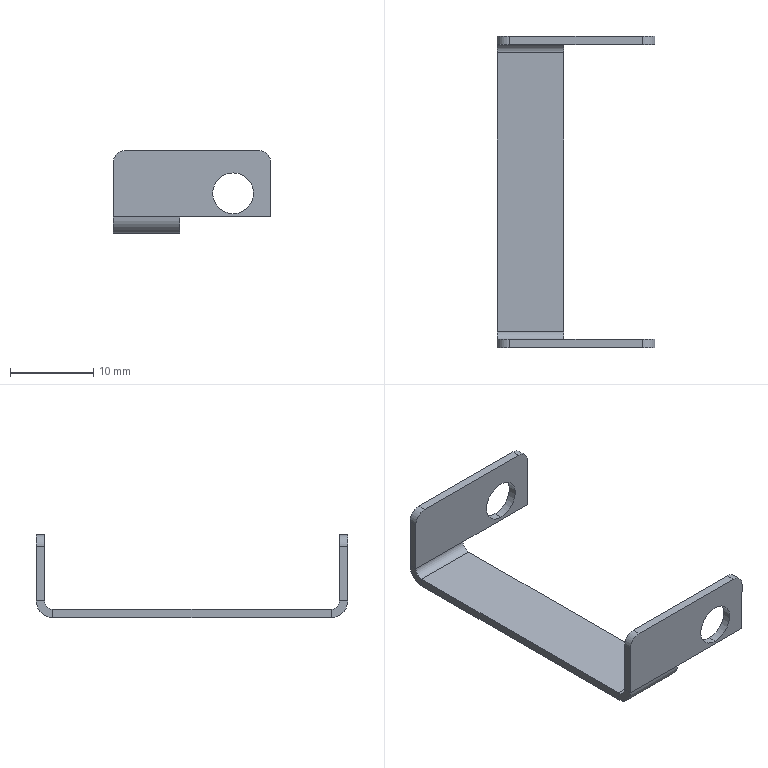Part | SolidWorks | features EdgeFlange 2, ICE 2, CornerTrim 1, FlatPattern 1, SMBaseFlange 1, SheetMetal 1 | 1 solid | 30 faces | box 19 x 37.5 x 10 mm | volume 570.053 mm3 | plane 18 | cylinder 12 | commonest cylinder face diameters 3 x4 4.9 x4 2 x2 4 x2
STEP:
#1=CARTESIAN_POINT('',(4.95,-17.75,6.3));
#2=VERTEX_POINT('',#1);
#3=CARTESIAN_POINT('',(4.95,-17.75,1.4));
#4=VERTEX_POINT('',#3);
#5=CARTESIAN_POINT('',(4.95,-17.75,3.85));
#6=DIRECTION('',(0.,-1.,0.));
#7=DIRECTION('',(0.,0.,-1.));
#8=AXIS2_PLACEMENT_3D('',#5,#6,#7);
#9=CIRCLE('',#8,2.45);
#10=EDGE_CURVE('',#2,#4,#9,.T.);
#11=ORIENTED_EDGE('',*,*,#10,.F.);
#12=CARTESIAN_POINT('',(4.95,-18.75,6.3));
#13=VERTEX_POINT('',#12);
#14=CARTESIAN_POINT('',(4.95,18.75,6.3));
#15=DIRECTION('',(0.,-1.,0.));
#16=VECTOR('',#15,1000.);
#17=LINE('',#14,#16);
#18=EDGE_CURVE('',#2,#13,#17,.T.);
#19=ORIENTED_EDGE('',*,*,#18,.T.);
#20=CARTESIAN_POINT('',(4.95,-18.75,1.4));
#21=VERTEX_POINT('',#20);
#22=CARTESIAN_POINT('',(4.95,-18.75,3.85));
#23=DIRECTION('',(0.,-1.,0.));
#24=DIRECTION('',(0.,0.,-1.));
#25=AXIS2_PLACEMENT_3D('',#22,#23,#24);
#26=CIRCLE('',#25,2.45);
#27=EDGE_CURVE('',#13,#21,#26,.T.);
#28=ORIENTED_EDGE('',*,*,#27,.T.);
#29=CARTESIAN_POINT('',(4.95,18.75,1.4));
#30=DIRECTION('',(0.,-1.,0.));
#31=VECTOR('',#30,1000.);
#32=LINE('',#29,#31);
#33=EDGE_CURVE('',#4,#21,#32,.T.);
#34=ORIENTED_EDGE('',*,*,#33,.F.);
#35=EDGE_LOOP('',(#11,#19,#28,#34));
#36=FACE_OUTER_BOUND('',#35,.T.);
#37=CARTESIAN_POINT('',(4.95,18.75,3.85));
#38=DIRECTION('',(0.,-1.,0.));
#39=DIRECTION('',(0.,0.,-1.));
#40=AXIS2_PLACEMENT_3D('',#37,#38,#39);
#41=CYLINDRICAL_SURFACE('',#40,2.45);
#42=ADVANCED_FACE('',(#36),#41,.F.);
#43=CARTESIAN_POINT('',(4.95,18.75,6.3));
#44=VERTEX_POINT('',#43);
#45=CARTESIAN_POINT('',(4.95,18.75,1.4));
#46=VERTEX_POINT('',#45);
#47=CARTESIAN_POINT('',(4.95,18.75,3.85));
#48=DIRECTION('',(0.,-1.,0.));
#49=DIRECTION('',(0.,0.,-1.));
#50=AXIS2_PLACEMENT_3D('',#47,#48,#49);
#51=CIRCLE('',#50,2.45);
#52=EDGE_CURVE('',#44,#46,#51,.T.);
#53=ORIENTED_EDGE('',*,*,#52,.F.);
#54=CARTESIAN_POINT('',(4.95,17.75,6.3));
#55=VERTEX_POINT('',#54);
#56=CARTESIAN_POINT('',(4.95,18.75,6.3));
#57=DIRECTION('',(0.,-1.,0.));
#58=VECTOR('',#57,1000.);
#59=LINE('',#56,#58);
#60=EDGE_CURVE('',#44,#55,#59,.T.);
#61=ORIENTED_EDGE('',*,*,#60,.T.);
#62=CARTESIAN_POINT('',(4.95,17.75,1.4));
#63=VERTEX_POINT('',#62);
#64=CARTESIAN_POINT('',(4.95,17.75,3.85));
#65=DIRECTION('',(0.,1.,0.));
#66=DIRECTION('',(0.,0.,1.));
#67=AXIS2_PLACEMENT_3D('',#64,#65,#66);
#68=CIRCLE('',#67,2.45);
#69=EDGE_CURVE('',#63,#55,#68,.T.);
#70=ORIENTED_EDGE('',*,*,#69,.F.);
#71=CARTESIAN_POINT('',(4.95,18.75,1.4));
#72=DIRECTION('',(0.,-1.,0.));
#73=VECTOR('',#72,1000.);
#74=LINE('',#71,#73);
#75=EDGE_CURVE('',#46,#63,#74,.T.);
#76=ORIENTED_EDGE('',*,*,#75,.F.);
#77=EDGE_LOOP('',(#53,#61,#70,#76));
#78=FACE_OUTER_BOUND('',#77,.T.);
#79=CARTESIAN_POINT('',(4.95,18.75,3.85));
#80=DIRECTION('',(0.,-1.,0.));
#81=DIRECTION('',(0.,0.,-1.));
#82=AXIS2_PLACEMENT_3D('',#79,#80,#81);
#83=CYLINDRICAL_SURFACE('',#82,2.45);
#84=ADVANCED_FACE('',(#78),#83,.F.);
#85=CARTESIAN_POINT('',(-1.5,-16.75,-1.));
#86=VERTEX_POINT('',#85);
#87=CARTESIAN_POINT('',(-1.5,16.75,-1.));
#88=VERTEX_POINT('',#87);
#89=CARTESIAN_POINT('',(-1.5,18.75,-1.));
#90=DIRECTION('',(0.,1.,0.));
#91=VECTOR('',#90,1000.);
#92=LINE('',#89,#91);
#93=EDGE_CURVE('',#86,#88,#92,.T.);
#94=ORIENTED_EDGE('',*,*,#93,.F.);
#95=CARTESIAN_POINT('',(-9.5,-16.75,-1.));
#96=VERTEX_POINT('',#95);
#97=CARTESIAN_POINT('',(9.5,-16.75,-1.));
#98=DIRECTION('',(-1.,0.,0.));
#99=VECTOR('',#98,1000.);
#100=LINE('',#97,#99);
#101=EDGE_CURVE('',#86,#96,#100,.T.);
#102=ORIENTED_EDGE('',*,*,#101,.T.);
#103=CARTESIAN_POINT('',(-9.5,16.75,-1.));
#104=VERTEX_POINT('',#103);
#105=CARTESIAN_POINT('',(-9.5,-18.75,-1.));
#106=DIRECTION('',(0.,-1.,0.));
#107=VECTOR('',#106,1000.);
#108=LINE('',#105,#107);
#109=EDGE_CURVE('',#104,#96,#108,.T.);
#110=ORIENTED_EDGE('',*,*,#109,.F.);
#111=CARTESIAN_POINT('',(-9.5,16.75,-1.));
#112=DIRECTION('',(1.,0.,0.));
#113=VECTOR('',#112,1000.);
#114=LINE('',#111,#113);
#115=EDGE_CURVE('',#104,#88,#114,.T.);
#116=ORIENTED_EDGE('',*,*,#115,.T.);
#117=EDGE_LOOP('',(#94,#102,#110,#116));
#118=FACE_OUTER_BOUND('',#117,.T.);
#119=CARTESIAN_POINT('',(0.,0.,-1.));
#120=DIRECTION('',(0.,0.,-1.));
#121=DIRECTION('',(-1.,0.,0.));
#122=AXIS2_PLACEMENT_3D('',#119,#120,#121);
#123=PLANE('',#122);
#124=ADVANCED_FACE('',(#118),#123,.T.);
#125=CARTESIAN_POINT('',(-1.5,-16.75,0.));
#126=VERTEX_POINT('',#125);
#127=CARTESIAN_POINT('',(-9.5,-16.75,0.));
#128=VERTEX_POINT('',#127);
#129=CARTESIAN_POINT('',(9.5,-16.75,0.));
#130=DIRECTION('',(-1.,0.,0.));
#131=VECTOR('',#130,1000.);
#132=LINE('',#129,#131);
#133=EDGE_CURVE('',#126,#128,#132,.T.);
#134=ORIENTED_EDGE('',*,*,#133,.F.);
#135=CARTESIAN_POINT('',(-1.5,16.75,0.));
#136=VERTEX_POINT('',#135);
#137=CARTESIAN_POINT('',(-1.5,0.,0.));
#138=DIRECTION('',(0.,1.,0.));
#139=VECTOR('',#138,1000.);
#140=LINE('',#137,#139);
#141=EDGE_CURVE('',#126,#136,#140,.T.);
#142=ORIENTED_EDGE('',*,*,#141,.T.);
#143=CARTESIAN_POINT('',(-9.5,16.75,0.));
#144=VERTEX_POINT('',#143);
#145=CARTESIAN_POINT('',(-9.5,16.75,0.));
#146=DIRECTION('',(1.,0.,0.));
#147=VECTOR('',#146,1000.);
#148=LINE('',#145,#147);
#149=EDGE_CURVE('',#144,#136,#148,.T.);
#150=ORIENTED_EDGE('',*,*,#149,.F.);
#151=CARTESIAN_POINT('',(-9.5,-18.75,0.));
#152=DIRECTION('',(0.,-1.,0.));
#153=VECTOR('',#152,1000.);
#154=LINE('',#151,#153);
#155=EDGE_CURVE('',#144,#128,#154,.T.);
#156=ORIENTED_EDGE('',*,*,#155,.T.);
#157=EDGE_LOOP('',(#134,#142,#150,#156));
#158=FACE_OUTER_BOUND('',#157,.T.);
#159=CARTESIAN_POINT('',(0.,0.,0.));
#160=DIRECTION('',(0.,0.,-1.));
#161=DIRECTION('',(-1.,0.,0.));
#162=AXIS2_PLACEMENT_3D('',#159,#160,#161);
#163=PLANE('',#162);
#164=ADVANCED_FACE('',(#158),#163,.F.);
#165=ORIENTED_EDGE('',*,*,#155,.F.);
#166=CARTESIAN_POINT('',(-9.5,16.75,0.));
#167=DIRECTION('',(0.,0.,-1.));
#168=VECTOR('',#167,1000.);
#169=LINE('',#166,#168);
#170=EDGE_CURVE('',#144,#104,#169,.T.);
#171=ORIENTED_EDGE('',*,*,#170,.T.);
#172=ORIENTED_EDGE('',*,*,#109,.T.);
#173=CARTESIAN_POINT('',(-9.5,-16.75,0.));
#174=DIRECTION('',(0.,0.,-1.));
#175=VECTOR('',#174,1000.);
#176=LINE('',#173,#175);
#177=EDGE_CURVE('',#128,#96,#176,.T.);
#178=ORIENTED_EDGE('',*,*,#177,.F.);
#179=EDGE_LOOP('',(#165,#171,#172,#178));
#180=FACE_OUTER_BOUND('',#179,.T.);
#181=CARTESIAN_POINT('',(-9.5,-18.75,-1.));
#182=DIRECTION('',(-1.,0.,0.));
#183=DIRECTION('',(0.,0.,1.));
#184=AXIS2_PLACEMENT_3D('',#181,#182,#183);
#185=PLANE('',#184);
#186=ADVANCED_FACE('',(#180),#185,.T.);
#187=CARTESIAN_POINT('',(-9.5,-17.75,1.));
#188=VERTEX_POINT('',#187);
#189=CARTESIAN_POINT('',(-9.5,-18.75,1.));
#190=VERTEX_POINT('',#189);
#191=CARTESIAN_POINT('',(-9.5,-18.75,1.));
#192=DIRECTION('',(0.,-1.,0.));
#193=VECTOR('',#192,1000.);
#194=LINE('',#191,#193);
#195=EDGE_CURVE('',#188,#190,#194,.T.);
#196=ORIENTED_EDGE('',*,*,#195,.F.);
#197=CARTESIAN_POINT('',(-9.5,-16.75,1.));
#198=DIRECTION('',(-1.,0.,0.));
#199=DIRECTION('',(0.,0.,-1.));
#200=AXIS2_PLACEMENT_3D('',#197,#198,#199);
#201=CIRCLE('',#200,1.);
#202=EDGE_CURVE('',#128,#188,#201,.T.);
#203=ORIENTED_EDGE('',*,*,#202,.F.);
#204=ORIENTED_EDGE('',*,*,#177,.T.);
#205=CARTESIAN_POINT('',(-9.5,-16.75,1.));
#206=DIRECTION('',(-1.,0.,0.));
#207=DIRECTION('',(0.,0.,-1.));
#208=AXIS2_PLACEMENT_3D('',#205,#206,#207);
#209=CIRCLE('',#208,2.);
#210=EDGE_CURVE('',#96,#190,#209,.T.);
#211=ORIENTED_EDGE('',*,*,#210,.T.);
#212=EDGE_LOOP('',(#196,#203,#204,#211));
#213=FACE_OUTER_BOUND('',#212,.T.);
#214=CARTESIAN_POINT('',(-9.5,-16.75,1.));
#215=DIRECTION('',(-1.,0.,0.));
#216=DIRECTION('',(0.,0.,1.));
#217=AXIS2_PLACEMENT_3D('',#214,#215,#216);
#218=PLANE('',#217);
#219=ADVANCED_FACE('',(#213),#218,.T.);
#220=CARTESIAN_POINT('',(-1.5,-18.75,1.));
#221=VERTEX_POINT('',#220);
#222=CARTESIAN_POINT('',(-1.5,-16.75,1.));
#223=DIRECTION('',(1.,0.,0.));
#224=DIRECTION('',(0.,-1.,0.));
#225=AXIS2_PLACEMENT_3D('',#222,#223,#224);
#226=CIRCLE('',#225,2.);
#227=EDGE_CURVE('',#221,#86,#226,.T.);
#228=ORIENTED_EDGE('',*,*,#227,.F.);
#229=CARTESIAN_POINT('',(0.,-18.75,1.));
#230=DIRECTION('',(1.,0.,0.));
#231=VECTOR('',#230,1000.);
#232=LINE('',#229,#231);
#233=EDGE_CURVE('',#190,#221,#232,.T.);
#234=ORIENTED_EDGE('',*,*,#233,.F.);
#235=ORIENTED_EDGE('',*,*,#210,.F.);
#236=ORIENTED_EDGE('',*,*,#101,.F.);
#237=EDGE_LOOP('',(#228,#234,#235,#236));
#238=FACE_OUTER_BOUND('',#237,.T.);
#239=CARTESIAN_POINT('',(9.5,-16.75,1.));
#240=DIRECTION('',(1.,0.,0.));
#241=DIRECTION('',(0.,-1.,0.));
#242=AXIS2_PLACEMENT_3D('',#239,#240,#241);
#243=CYLINDRICAL_SURFACE('',#242,2.);
#244=ADVANCED_FACE('',(#238),#243,.T.);
#245=CARTESIAN_POINT('',(-1.5,-17.75,1.));
#246=VERTEX_POINT('',#245);
#247=CARTESIAN_POINT('',(-9.5,-17.75,1.));
#248=DIRECTION('',(1.,0.,0.));
#249=VECTOR('',#248,1000.);
#250=LINE('',#247,#249);
#251=EDGE_CURVE('',#188,#246,#250,.T.);
#252=ORIENTED_EDGE('',*,*,#251,.T.);
#253=CARTESIAN_POINT('',(-1.5,-16.75,1.));
#254=DIRECTION('',(1.,0.,0.));
#255=DIRECTION('',(0.,-1.,0.));
#256=AXIS2_PLACEMENT_3D('',#253,#254,#255);
#257=CIRCLE('',#256,1.);
#258=EDGE_CURVE('',#246,#126,#257,.T.);
#259=ORIENTED_EDGE('',*,*,#258,.T.);
#260=ORIENTED_EDGE('',*,*,#133,.T.);
#261=ORIENTED_EDGE('',*,*,#202,.T.);
#262=EDGE_LOOP('',(#252,#259,#260,#261));
#263=FACE_OUTER_BOUND('',#262,.T.);
#264=CARTESIAN_POINT('',(9.5,-16.75,1.));
#265=DIRECTION('',(1.,0.,0.));
#266=DIRECTION('',(0.,-1.,0.));
#267=AXIS2_PLACEMENT_3D('',#264,#265,#266);
#268=CYLINDRICAL_SURFACE('',#267,1.);
#269=ADVANCED_FACE('',(#263),#268,.F.);
#270=CARTESIAN_POINT('',(9.5,-17.75,7.5));
#271=VERTEX_POINT('',#270);
#272=CARTESIAN_POINT('',(9.5,-17.75,1.));
#273=VERTEX_POINT('',#272);
#274=CARTESIAN_POINT('',(9.5,-17.75,0.));
#275=DIRECTION('',(0.,0.,-1.));
#276=VECTOR('',#275,1000.);
#277=LINE('',#274,#276);
#278=EDGE_CURVE('',#271,#273,#277,.T.);
#279=ORIENTED_EDGE('',*,*,#278,.F.);
#280=CARTESIAN_POINT('',(9.5,-18.75,7.5));
#281=VERTEX_POINT('',#280);
#282=CARTESIAN_POINT('',(9.5,-18.75,7.5));
#283=DIRECTION('',(0.,-1.,0.));
#284=VECTOR('',#283,1000.);
#285=LINE('',#282,#284);
#286=EDGE_CURVE('',#271,#281,#285,.T.);
#287=ORIENTED_EDGE('',*,*,#286,.T.);
#288=CARTESIAN_POINT('',(9.5,-18.75,1.));
#289=VERTEX_POINT('',#288);
#290=CARTESIAN_POINT('',(9.5,-18.75,0.));
#291=DIRECTION('',(0.,0.,-1.));
#292=VECTOR('',#291,1000.);
#293=LINE('',#290,#292);
#294=EDGE_CURVE('',#281,#289,#293,.T.);
#295=ORIENTED_EDGE('',*,*,#294,.T.);
#296=CARTESIAN_POINT('',(9.5,-17.75,1.));
#297=DIRECTION('',(0.,-1.,0.));
#298=VECTOR('',#297,1000.);
#299=LINE('',#296,#298);
#300=EDGE_CURVE('',#273,#289,#299,.T.);
#301=ORIENTED_EDGE('',*,*,#300,.F.);
#302=EDGE_LOOP('',(#279,#287,#295,#301));
#303=FACE_OUTER_BOUND('',#302,.T.);
#304=CARTESIAN_POINT('',(9.5,-18.75,0.));
#305=DIRECTION('',(1.,0.,0.));
#306=DIRECTION('',(0.,0.,-1.));
#307=AXIS2_PLACEMENT_3D('',#304,#305,#306);
#308=PLANE('',#307);
#309=ADVANCED_FACE('',(#303),#308,.T.);
#310=CARTESIAN_POINT('',(-9.5,-18.75,7.5));
#311=VERTEX_POINT('',#310);
#312=CARTESIAN_POINT('',(-9.5,-18.75,9.));
#313=DIRECTION('',(0.,0.,1.));
#314=VECTOR('',#313,1000.);
#315=LINE('',#312,#314);
#316=EDGE_CURVE('',#190,#311,#315,.T.);
#317=ORIENTED_EDGE('',*,*,#316,.T.);
#318=CARTESIAN_POINT('',(-9.5,-17.75,7.5));
#319=VERTEX_POINT('',#318);
#320=CARTESIAN_POINT('',(-9.5,-18.75,7.5));
#321=DIRECTION('',(0.,1.,0.));
#322=VECTOR('',#321,1000.);
#323=LINE('',#320,#322);
#324=EDGE_CURVE('',#311,#319,#323,.T.);
#325=ORIENTED_EDGE('',*,*,#324,.T.);
#326=CARTESIAN_POINT('',(-9.5,-17.75,0.));
#327=DIRECTION('',(0.,0.,1.));
#328=VECTOR('',#327,1000.);
#329=LINE('',#326,#328);
#330=EDGE_CURVE('',#188,#319,#329,.T.);
#331=ORIENTED_EDGE('',*,*,#330,.F.);
#332=ORIENTED_EDGE('',*,*,#195,.T.);
#333=EDGE_LOOP('',(#317,#325,#331,#332));
#334=FACE_OUTER_BOUND('',#333,.T.);
#335=CARTESIAN_POINT('',(-9.5,-18.75,9.));
#336=DIRECTION('',(-1.,0.,0.));
#337=DIRECTION('',(0.,0.,1.));
#338=AXIS2_PLACEMENT_3D('',#335,#336,#337);
#339=PLANE('',#338);
#340=ADVANCED_FACE('',(#334),#339,.T.);
#341=CARTESIAN_POINT('',(4.95,-18.75,3.85));
#342=DIRECTION('',(0.,-1.,0.));
#343=DIRECTION('',(0.,0.,-1.));
#344=AXIS2_PLACEMENT_3D('',#341,#342,#343);
#345=CIRCLE('',#344,2.45);
#346=EDGE_CURVE('',#21,#13,#345,.T.);
#347=ORIENTED_EDGE('',*,*,#346,.F.);
#348=ORIENTED_EDGE('',*,*,#27,.F.);
#349=EDGE_LOOP('',(#347,#348));
#350=FACE_BOUND('',#349,.T.);
#351=CARTESIAN_POINT('',(-8.,-18.75,9.));
#352=VERTEX_POINT('',#351);
#353=CARTESIAN_POINT('',(8.,-18.75,9.));
#354=VERTEX_POINT('',#353);
#355=CARTESIAN_POINT('',(9.5,-18.75,9.));
#356=DIRECTION('',(1.,0.,0.));
#357=VECTOR('',#356,1000.);
#358=LINE('',#355,#357);
#359=EDGE_CURVE('',#352,#354,#358,.T.);
#360=ORIENTED_EDGE('',*,*,#359,.F.);
#361=CARTESIAN_POINT('',(-8.,-18.75,7.5));
#362=DIRECTION('',(0.,-1.,0.));
#363=DIRECTION('',(0.,0.,-1.));
#364=AXIS2_PLACEMENT_3D('',#361,#362,#363);
#365=CIRCLE('',#364,1.5);
#366=EDGE_CURVE('',#352,#311,#365,.T.);
#367=ORIENTED_EDGE('',*,*,#366,.T.);
#368=ORIENTED_EDGE('',*,*,#316,.F.);
#369=ORIENTED_EDGE('',*,*,#233,.T.);
#370=CARTESIAN_POINT('',(-1.5,-18.75,1.));
#371=DIRECTION('',(-1.,0.,0.));
#372=VECTOR('',#371,1000.);
#373=LINE('',#370,#372);
#374=EDGE_CURVE('',#289,#221,#373,.T.);
#375=ORIENTED_EDGE('',*,*,#374,.F.);
#376=ORIENTED_EDGE('',*,*,#294,.F.);
#377=CARTESIAN_POINT('',(8.,-18.75,7.5));
#378=DIRECTION('',(0.,-1.,0.));
#379=DIRECTION('',(0.,0.,-1.));
#380=AXIS2_PLACEMENT_3D('',#377,#378,#379);
#381=CIRCLE('',#380,1.5);
#382=EDGE_CURVE('',#281,#354,#381,.T.);
#383=ORIENTED_EDGE('',*,*,#382,.T.);
#384=EDGE_LOOP('',(#360,#367,#368,#369,#375,#376,#383));
#385=FACE_OUTER_BOUND('',#384,.T.);
#386=CARTESIAN_POINT('',(0.,-18.75,0.));
#387=DIRECTION('',(0.,-1.,0.));
#388=DIRECTION('',(0.,0.,-1.));
#389=AXIS2_PLACEMENT_3D('',#386,#387,#388);
#390=PLANE('',#389);
#391=ADVANCED_FACE('',(#350,#385),#390,.T.);
#392=CARTESIAN_POINT('',(4.95,-17.75,3.85));
#393=DIRECTION('',(0.,-1.,0.));
#394=DIRECTION('',(0.,0.,-1.));
#395=AXIS2_PLACEMENT_3D('',#392,#393,#394);
#396=CIRCLE('',#395,2.45);
#397=EDGE_CURVE('',#4,#2,#396,.T.);
#398=ORIENTED_EDGE('',*,*,#397,.T.);
#399=ORIENTED_EDGE('',*,*,#10,.T.);
#400=EDGE_LOOP('',(#398,#399));
#401=FACE_BOUND('',#400,.T.);
#402=ORIENTED_EDGE('',*,*,#330,.T.);
#403=CARTESIAN_POINT('',(-8.,-17.75,9.));
#404=VERTEX_POINT('',#403);
#405=CARTESIAN_POINT('',(-8.,-17.75,7.5));
#406=DIRECTION('',(0.,1.,0.));
#407=DIRECTION('',(0.,0.,-1.));
#408=AXIS2_PLACEMENT_3D('',#405,#406,#407);
#409=CIRCLE('',#408,1.5);
#410=EDGE_CURVE('',#319,#404,#409,.T.);
#411=ORIENTED_EDGE('',*,*,#410,.T.);
#412=CARTESIAN_POINT('',(8.,-17.75,9.));
#413=VERTEX_POINT('',#412);
#414=CARTESIAN_POINT('',(0.,-17.75,9.));
#415=DIRECTION('',(1.,0.,0.));
#416=VECTOR('',#415,1000.);
#417=LINE('',#414,#416);
#418=EDGE_CURVE('',#404,#413,#417,.T.);
#419=ORIENTED_EDGE('',*,*,#418,.T.);
#420=CARTESIAN_POINT('',(8.,-17.75,7.5));
#421=DIRECTION('',(0.,1.,0.));
#422=DIRECTION('',(0.,0.,-1.));
#423=AXIS2_PLACEMENT_3D('',#420,#421,#422);
#424=CIRCLE('',#423,1.5);
#425=EDGE_CURVE('',#413,#271,#424,.T.);
#426=ORIENTED_EDGE('',*,*,#425,.T.);
#427=ORIENTED_EDGE('',*,*,#278,.T.);
#428=CARTESIAN_POINT('',(0.,-17.75,1.));
#429=DIRECTION('',(-1.,0.,0.));
#430=VECTOR('',#429,1000.);
#431=LINE('',#428,#430);
#432=EDGE_CURVE('',#273,#246,#431,.T.);
#433=ORIENTED_EDGE('',*,*,#432,.T.);
#434=ORIENTED_EDGE('',*,*,#251,.F.);
#435=EDGE_LOOP('',(#402,#411,#419,#426,#427,#433,#434));
#436=FACE_OUTER_BOUND('',#435,.T.);
#437=CARTESIAN_POINT('',(0.,-17.75,0.));
#438=DIRECTION('',(0.,-1.,0.));
#439=DIRECTION('',(0.,0.,-1.));
#440=AXIS2_PLACEMENT_3D('',#437,#438,#439);
#441=PLANE('',#440);
#442=ADVANCED_FACE('',(#401,#436),#441,.F.);
#443=ORIENTED_EDGE('',*,*,#418,.F.);
#444=CARTESIAN_POINT('',(-8.,-18.75,9.));
#445=DIRECTION('',(0.,-1.,0.));
#446=VECTOR('',#445,1000.);
#447=LINE('',#444,#446);
#448=EDGE_CURVE('',#404,#352,#447,.T.);
#449=ORIENTED_EDGE('',*,*,#448,.T.);
#450=ORIENTED_EDGE('',*,*,#359,.T.);
#451=CARTESIAN_POINT('',(8.,-18.75,9.));
#452=DIRECTION('',(0.,1.,0.));
#453=VECTOR('',#452,1000.);
#454=LINE('',#451,#453);
#455=EDGE_CURVE('',#354,#413,#454,.T.);
#456=ORIENTED_EDGE('',*,*,#455,.T.);
#457=EDGE_LOOP('',(#443,#449,#450,#456));
#458=FACE_OUTER_BOUND('',#457,.T.);
#459=CARTESIAN_POINT('',(9.5,-18.75,9.));
#460=DIRECTION('',(0.,0.,1.));
#461=DIRECTION('',(0.,-1.,0.));
#462=AXIS2_PLACEMENT_3D('',#459,#460,#461);
#463=PLANE('',#462);
#464=ADVANCED_FACE('',(#458),#463,.T.);
#465=CARTESIAN_POINT('',(-9.5,17.75,1.));
#466=VERTEX_POINT('',#465);
#467=CARTESIAN_POINT('',(-9.5,16.75,1.));
#468=DIRECTION('',(-1.,0.,0.));
#469=DIRECTION('',(0.,0.,1.));
#470=AXIS2_PLACEMENT_3D('',#467,#468,#469);
#471=CIRCLE('',#470,1.);
#472=EDGE_CURVE('',#466,#144,#471,.T.);
#473=ORIENTED_EDGE('',*,*,#472,.F.);
#474=CARTESIAN_POINT('',(-9.5,18.75,1.));
#475=VERTEX_POINT('',#474);
#476=CARTESIAN_POINT('',(-9.5,17.75,1.));
#477=DIRECTION('',(0.,1.,0.));
#478=VECTOR('',#477,1000.);
#479=LINE('',#476,#478);
#480=EDGE_CURVE('',#466,#475,#479,.T.);
#481=ORIENTED_EDGE('',*,*,#480,.T.);
#482=CARTESIAN_POINT('',(-9.5,16.75,1.));
#483=DIRECTION('',(-1.,0.,0.));
#484=DIRECTION('',(0.,0.,1.));
#485=AXIS2_PLACEMENT_3D('',#482,#483,#484);
#486=CIRCLE('',#485,2.);
#487=EDGE_CURVE('',#475,#104,#486,.T.);
#488=ORIENTED_EDGE('',*,*,#487,.T.);
#489=ORIENTED_EDGE('',*,*,#170,.F.);
#490=EDGE_LOOP('',(#473,#481,#488,#489));
#491=FACE_OUTER_BOUND('',#490,.T.);
#492=CARTESIAN_POINT('',(-9.5,16.75,1.));
#493=DIRECTION('',(1.,0.,0.));
#494=DIRECTION('',(0.,0.,-1.));
#495=AXIS2_PLACEMENT_3D('',#492,#493,#494);
#496=PLANE('',#495);
#497=ADVANCED_FACE('',(#491),#496,.F.);
#498=CARTESIAN_POINT('',(-1.5,18.75,1.));
#499=VERTEX_POINT('',#498);
#500=CARTESIAN_POINT('',(-1.5,16.75,1.));
#501=DIRECTION('',(1.,0.,0.));
#502=DIRECTION('',(0.,-1.,0.));
#503=AXIS2_PLACEMENT_3D('',#500,#501,#502);
#504=CIRCLE('',#503,2.);
#505=EDGE_CURVE('',#88,#499,#504,.T.);
#506=ORIENTED_EDGE('',*,*,#505,.F.);
#507=ORIENTED_EDGE('',*,*,#115,.F.);
#508=ORIENTED_EDGE('',*,*,#487,.F.);
#509=CARTESIAN_POINT('',(0.,18.75,1.));
#510=DIRECTION('',(-1.,0.,0.));
#511=VECTOR('',#510,1000.);
#512=LINE('',#509,#511);
#513=EDGE_CURVE('',#499,#475,#512,.T.);
#514=ORIENTED_EDGE('',*,*,#513,.F.);
#515=EDGE_LOOP('',(#506,#507,#508,#514));
#516=FACE_OUTER_BOUND('',#515,.T.);
#517=CARTESIAN_POINT('',(-9.5,16.75,1.));
#518=DIRECTION('',(-1.,0.,0.));
#519=DIRECTION('',(0.,1.,0.));
#520=AXIS2_PLACEMENT_3D('',#517,#518,#519);
#521=CYLINDRICAL_SURFACE('',#520,2.);
#522=ADVANCED_FACE('',(#516),#521,.T.);
#523=ORIENTED_EDGE('',*,*,#149,.T.);
#524=CARTESIAN_POINT('',(-1.5,17.75,1.));
#525=VERTEX_POINT('',#524);
#526=CARTESIAN_POINT('',(-1.5,16.75,1.));
#527=DIRECTION('',(1.,0.,0.));
#528=DIRECTION('',(0.,-1.,0.));
#529=AXIS2_PLACEMENT_3D('',#526,#527,#528);
#530=CIRCLE('',#529,1.);
#531=EDGE_CURVE('',#136,#525,#530,.T.);
#532=ORIENTED_EDGE('',*,*,#531,.T.);
#533=CARTESIAN_POINT('',(9.5,17.75,1.));
#534=DIRECTION('',(-1.,0.,0.));
#535=VECTOR('',#534,1000.);
#536=LINE('',#533,#535);
#537=EDGE_CURVE('',#525,#466,#536,.T.);
#538=ORIENTED_EDGE('',*,*,#537,.T.);
#539=ORIENTED_EDGE('',*,*,#472,.T.);
#540=EDGE_LOOP('',(#523,#532,#538,#539));
#541=FACE_OUTER_BOUND('',#540,.T.);
#542=CARTESIAN_POINT('',(-9.5,16.75,1.));
#543=DIRECTION('',(-1.,0.,0.));
#544=DIRECTION('',(0.,1.,0.));
#545=AXIS2_PLACEMENT_3D('',#542,#543,#544);
#546=CYLINDRICAL_SURFACE('',#545,1.);
#547=ADVANCED_FACE('',(#541),#546,.F.);
#548=CARTESIAN_POINT('',(-9.5,17.75,7.5));
#549=VERTEX_POINT('',#548);
#550=CARTESIAN_POINT('',(-9.5,17.75,0.));
#551=DIRECTION('',(0.,0.,-1.));
#552=VECTOR('',#551,1000.);
#553=LINE('',#550,#552);
#554=EDGE_CURVE('',#549,#466,#553,.T.);
#555=ORIENTED_EDGE('',*,*,#554,.F.);
#556=CARTESIAN_POINT('',(-9.5,18.75,7.5));
#557=VERTEX_POINT('',#556);
#558=CARTESIAN_POINT('',(-9.5,18.75,7.5));
#559=DIRECTION('',(0.,1.,0.));
#560=VECTOR('',#559,1000.);
#561=LINE('',#558,#560);
#562=EDGE_CURVE('',#549,#557,#561,.T.);
#563=ORIENTED_EDGE('',*,*,#562,.T.);
#564=CARTESIAN_POINT('',(-9.5,18.75,0.));
#565=DIRECTION('',(0.,0.,-1.));
#566=VECTOR('',#565,1000.);
#567=LINE('',#564,#566);
#568=EDGE_CURVE('',#557,#475,#567,.T.);
#569=ORIENTED_EDGE('',*,*,#568,.T.);
#570=ORIENTED_EDGE('',*,*,#480,.F.);
#571=EDGE_LOOP('',(#555,#563,#569,#570));
#572=FACE_OUTER_BOUND('',#571,.T.);
#573=CARTESIAN_POINT('',(-9.5,18.75,0.));
#574=DIRECTION('',(-1.,0.,0.));
#575=DIRECTION('',(0.,0.,1.));
#576=AXIS2_PLACEMENT_3D('',#573,#574,#575);
#577=PLANE('',#576);
#578=ADVANCED_FACE('',(#572),#577,.T.);
#579=CARTESIAN_POINT('',(9.5,18.75,1.));
#580=VERTEX_POINT('',#579);
#581=CARTESIAN_POINT('',(9.5,18.75,7.5));
#582=VERTEX_POINT('',#581);
#583=CARTESIAN_POINT('',(9.5,18.75,9.));
#584=DIRECTION('',(0.,0.,1.));
#585=VECTOR('',#584,1000.);
#586=LINE('',#583,#585);
#587=EDGE_CURVE('',#580,#582,#586,.T.);
#588=ORIENTED_EDGE('',*,*,#587,.T.);
#589=CARTESIAN_POINT('',(9.5,17.75,7.5));
#590=VERTEX_POINT('',#589);
#591=CARTESIAN_POINT('',(9.5,18.75,7.5));
#592=DIRECTION('',(0.,-1.,0.));
#593=VECTOR('',#592,1000.);
#594=LINE('',#591,#593);
#595=EDGE_CURVE('',#582,#590,#594,.T.);
#596=ORIENTED_EDGE('',*,*,#595,.T.);
#597=CARTESIAN_POINT('',(9.5,17.75,1.));
#598=VERTEX_POINT('',#597);
#599=CARTESIAN_POINT('',(9.5,17.75,0.));
#600=DIRECTION('',(0.,0.,1.));
#601=VECTOR('',#600,1000.);
#602=LINE('',#599,#601);
#603=EDGE_CURVE('',#598,#590,#602,.T.);
#604=ORIENTED_EDGE('',*,*,#603,.F.);
#605=CARTESIAN_POINT('',(9.5,18.75,1.));
#606=DIRECTION('',(0.,1.,0.));
#607=VECTOR('',#606,1000.);
#608=LINE('',#605,#607);
#609=EDGE_CURVE('',#598,#580,#608,.T.);
#610=ORIENTED_EDGE('',*,*,#609,.T.);
#611=EDGE_LOOP('',(#588,#596,#604,#610));
#612=FACE_OUTER_BOUND('',#611,.T.);
#613=CARTESIAN_POINT('',(9.5,18.75,9.));
#614=DIRECTION('',(1.,0.,0.));
#615=DIRECTION('',(0.,0.,-1.));
#616=AXIS2_PLACEMENT_3D('',#613,#614,#615);
#617=PLANE('',#616);
#618=ADVANCED_FACE('',(#612),#617,.T.);
#619=CARTESIAN_POINT('',(4.95,18.75,3.85));
#620=DIRECTION('',(0.,-1.,0.));
#621=DIRECTION('',(0.,0.,-1.));
#622=AXIS2_PLACEMENT_3D('',#619,#620,#621);
#623=CIRCLE('',#622,2.45);
#624=EDGE_CURVE('',#46,#44,#623,.T.);
#625=ORIENTED_EDGE('',*,*,#624,.T.);
#626=ORIENTED_EDGE('',*,*,#52,.T.);
#627=EDGE_LOOP('',(#625,#626));
#628=FACE_BOUND('',#627,.T.);
#629=ORIENTED_EDGE('',*,*,#568,.F.);
#630=CARTESIAN_POINT('',(-8.,18.75,9.));
#631=VERTEX_POINT('',#630);
#632=CARTESIAN_POINT('',(-8.,18.75,7.5));
#633=DIRECTION('',(0.,1.,0.));
#634=DIRECTION('',(0.,0.,1.));
#635=AXIS2_PLACEMENT_3D('',#632,#633,#634);
#636=CIRCLE('',#635,1.5);
#637=EDGE_CURVE('',#557,#631,#636,.T.);
#638=ORIENTED_EDGE('',*,*,#637,.T.);
#639=CARTESIAN_POINT('',(8.,18.75,9.));
#640=VERTEX_POINT('',#639);
#641=CARTESIAN_POINT('',(-9.5,18.75,9.));
#642=DIRECTION('',(-1.,0.,0.));
#643=VECTOR('',#642,1000.);
#644=LINE('',#641,#643);
#645=EDGE_CURVE('',#640,#631,#644,.T.);
#646=ORIENTED_EDGE('',*,*,#645,.F.);
#647=CARTESIAN_POINT('',(8.,18.75,7.5));
#648=DIRECTION('',(0.,1.,0.));
#649=DIRECTION('',(0.,0.,1.));
#650=AXIS2_PLACEMENT_3D('',#647,#648,#649);
#651=CIRCLE('',#650,1.5);
#652=EDGE_CURVE('',#640,#582,#651,.T.);
#653=ORIENTED_EDGE('',*,*,#652,.T.);
#654=ORIENTED_EDGE('',*,*,#587,.F.);
#655=CARTESIAN_POINT('',(0.,18.75,1.));
#656=DIRECTION('',(-1.,0.,0.));
#657=VECTOR('',#656,1000.);
#658=LINE('',#655,#657);
#659=EDGE_CURVE('',#580,#499,#658,.T.);
#660=ORIENTED_EDGE('',*,*,#659,.T.);
#661=ORIENTED_EDGE('',*,*,#513,.T.);
#662=EDGE_LOOP('',(#629,#638,#646,#653,#654,#660,#661));
#663=FACE_OUTER_BOUND('',#662,.T.);
#664=CARTESIAN_POINT('',(0.,18.75,0.));
#665=DIRECTION('',(0.,1.,0.));
#666=DIRECTION('',(0.,0.,1.));
#667=AXIS2_PLACEMENT_3D('',#664,#665,#666);
#668=PLANE('',#667);
#669=ADVANCED_FACE('',(#628,#663),#668,.T.);
#670=ORIENTED_EDGE('',*,*,#69,.T.);
#671=CARTESIAN_POINT('',(4.95,17.75,3.85));
#672=DIRECTION('',(0.,1.,0.));
#673=DIRECTION('',(0.,0.,1.));
#674=AXIS2_PLACEMENT_3D('',#671,#672,#673);
#675=CIRCLE('',#674,2.45);
#676=EDGE_CURVE('',#55,#63,#675,.T.);
#677=ORIENTED_EDGE('',*,*,#676,.T.);
#678=EDGE_LOOP('',(#670,#677));
#679=FACE_BOUND('',#678,.T.);
#680=CARTESIAN_POINT('',(8.,17.75,9.));
#681=VERTEX_POINT('',#680);
#682=CARTESIAN_POINT('',(-8.,17.75,9.));
#683=VERTEX_POINT('',#682);
#684=CARTESIAN_POINT('',(0.,17.75,9.));
#685=DIRECTION('',(-1.,0.,0.));
#686=VECTOR('',#685,1000.);
#687=LINE('',#684,#686);
#688=EDGE_CURVE('',#681,#683,#687,.T.);
#689=ORIENTED_EDGE('',*,*,#688,.T.);
#690=CARTESIAN_POINT('',(-8.,17.75,7.5));
#691=DIRECTION('',(0.,-1.,0.));
#692=DIRECTION('',(0.,0.,1.));
#693=AXIS2_PLACEMENT_3D('',#690,#691,#692);
#694=CIRCLE('',#693,1.5);
#695=EDGE_CURVE('',#683,#549,#694,.T.);
#696=ORIENTED_EDGE('',*,*,#695,.T.);
#697=ORIENTED_EDGE('',*,*,#554,.T.);
#698=ORIENTED_EDGE('',*,*,#537,.F.);
#699=CARTESIAN_POINT('',(9.5,17.75,1.));
#700=DIRECTION('',(-1.,0.,0.));
#701=VECTOR('',#700,1000.);
#702=LINE('',#699,#701);
#703=EDGE_CURVE('',#598,#525,#702,.T.);
#704=ORIENTED_EDGE('',*,*,#703,.F.);
#705=ORIENTED_EDGE('',*,*,#603,.T.);
#706=CARTESIAN_POINT('',(8.,17.75,7.5));
#707=DIRECTION('',(0.,-1.,0.));
#708=DIRECTION('',(0.,0.,1.));
#709=AXIS2_PLACEMENT_3D('',#706,#707,#708);
#710=CIRCLE('',#709,1.5);
#711=EDGE_CURVE('',#590,#681,#710,.T.);
#712=ORIENTED_EDGE('',*,*,#711,.T.);
#713=EDGE_LOOP('',(#689,#696,#697,#698,#704,#705,#712));
#714=FACE_OUTER_BOUND('',#713,.T.);
#715=CARTESIAN_POINT('',(0.,17.75,0.));
#716=DIRECTION('',(0.,1.,0.));
#717=DIRECTION('',(0.,0.,1.));
#718=AXIS2_PLACEMENT_3D('',#715,#716,#717);
#719=PLANE('',#718);
#720=ADVANCED_FACE('',(#679,#714),#719,.F.);
#721=ORIENTED_EDGE('',*,*,#645,.T.);
#722=CARTESIAN_POINT('',(-8.,18.75,9.));
#723=DIRECTION('',(0.,-1.,0.));
#724=VECTOR('',#723,1000.);
#725=LINE('',#722,#724);
#726=EDGE_CURVE('',#631,#683,#725,.T.);
#727=ORIENTED_EDGE('',*,*,#726,.T.);
#728=ORIENTED_EDGE('',*,*,#688,.F.);
#729=CARTESIAN_POINT('',(8.,18.75,9.));
#730=DIRECTION('',(0.,1.,0.));
#731=VECTOR('',#730,1000.);
#732=LINE('',#729,#731);
#733=EDGE_CURVE('',#681,#640,#732,.T.);
#734=ORIENTED_EDGE('',*,*,#733,.T.);
#735=EDGE_LOOP('',(#721,#727,#728,#734));
#736=FACE_OUTER_BOUND('',#735,.T.);
#737=CARTESIAN_POINT('',(-9.5,18.75,9.));
#738=DIRECTION('',(0.,0.,1.));
#739=DIRECTION('',(0.,-1.,0.));
#740=AXIS2_PLACEMENT_3D('',#737,#738,#739);
#741=PLANE('',#740);
#742=ADVANCED_FACE('',(#736),#741,.T.);
#743=ORIENTED_EDGE('',*,*,#227,.T.);
#744=ORIENTED_EDGE('',*,*,#93,.T.);
#745=ORIENTED_EDGE('',*,*,#505,.T.);
#746=CARTESIAN_POINT('',(-1.5,18.75,1.));
#747=DIRECTION('',(0.,1.,0.));
#748=VECTOR('',#747,1000.);
#749=LINE('',#746,#748);
#750=EDGE_CURVE('',#525,#499,#749,.T.);
#751=ORIENTED_EDGE('',*,*,#750,.F.);
#752=ORIENTED_EDGE('',*,*,#531,.F.);
#753=ORIENTED_EDGE('',*,*,#141,.F.);
#754=ORIENTED_EDGE('',*,*,#258,.F.);
#755=CARTESIAN_POINT('',(-1.5,18.75,1.));
#756=DIRECTION('',(0.,1.,0.));
#757=VECTOR('',#756,1000.);
#758=LINE('',#755,#757);
#759=EDGE_CURVE('',#221,#246,#758,.T.);
#760=ORIENTED_EDGE('',*,*,#759,.F.);
#761=EDGE_LOOP('',(#743,#744,#745,#751,#752,#753,#754,#760));
#762=FACE_OUTER_BOUND('',#761,.T.);
#763=CARTESIAN_POINT('',(-1.5,18.75,1.));
#764=DIRECTION('',(-1.,0.,0.));
#765=DIRECTION('',(0.,-1.,0.));
#766=AXIS2_PLACEMENT_3D('',#763,#764,#765);
#767=PLANE('',#766);
#768=ADVANCED_FACE('',(#762),#767,.F.);
#769=ORIENTED_EDGE('',*,*,#300,.T.);
#770=ORIENTED_EDGE('',*,*,#374,.T.);
#771=ORIENTED_EDGE('',*,*,#759,.T.);
#772=ORIENTED_EDGE('',*,*,#432,.F.);
#773=EDGE_LOOP('',(#769,#770,#771,#772));
#774=FACE_OUTER_BOUND('',#773,.T.);
#775=CARTESIAN_POINT('',(0.,0.,1.));
#776=DIRECTION('',(0.,0.,1.));
#777=DIRECTION('',(1.,0.,0.));
#778=AXIS2_PLACEMENT_3D('',#775,#776,#777);
#779=PLANE('',#778);
#780=ADVANCED_FACE('',(#774),#779,.F.);
#781=ORIENTED_EDGE('',*,*,#750,.T.);
#782=ORIENTED_EDGE('',*,*,#659,.F.);
#783=ORIENTED_EDGE('',*,*,#609,.F.);
#784=ORIENTED_EDGE('',*,*,#703,.T.);
#785=EDGE_LOOP('',(#781,#782,#783,#784));
#786=FACE_OUTER_BOUND('',#785,.T.);
#787=CARTESIAN_POINT('',(0.,0.,1.));
#788=DIRECTION('',(0.,0.,1.));
#789=DIRECTION('',(1.,0.,0.));
#790=AXIS2_PLACEMENT_3D('',#787,#788,#789);
#791=PLANE('',#790);
#792=ADVANCED_FACE('',(#786),#791,.F.);
#793=ORIENTED_EDGE('',*,*,#637,.F.);
#794=ORIENTED_EDGE('',*,*,#562,.F.);
#795=ORIENTED_EDGE('',*,*,#695,.F.);
#796=ORIENTED_EDGE('',*,*,#726,.F.);
#797=EDGE_LOOP('',(#793,#794,#795,#796));
#798=FACE_OUTER_BOUND('',#797,.T.);
#799=CARTESIAN_POINT('',(-8.,18.75,7.5));
#800=DIRECTION('',(0.,-1.,0.));
#801=DIRECTION('',(0.,0.,-1.));
#802=AXIS2_PLACEMENT_3D('',#799,#800,#801);
#803=CYLINDRICAL_SURFACE('',#802,1.5);
#804=ADVANCED_FACE('',(#798),#803,.T.);
#805=ORIENTED_EDGE('',*,*,#652,.F.);
#806=ORIENTED_EDGE('',*,*,#733,.F.);
#807=ORIENTED_EDGE('',*,*,#711,.F.);
#808=ORIENTED_EDGE('',*,*,#595,.F.);
#809=EDGE_LOOP('',(#805,#806,#807,#808));
#810=FACE_OUTER_BOUND('',#809,.T.);
#811=CARTESIAN_POINT('',(8.,18.75,7.5));
#812=DIRECTION('',(0.,-1.,0.));
#813=DIRECTION('',(0.,0.,-1.));
#814=AXIS2_PLACEMENT_3D('',#811,#812,#813);
#815=CYLINDRICAL_SURFACE('',#814,1.5);
#816=ADVANCED_FACE('',(#810),#815,.T.);
#817=ORIENTED_EDGE('',*,*,#366,.F.);
#818=ORIENTED_EDGE('',*,*,#448,.F.);
#819=ORIENTED_EDGE('',*,*,#410,.F.);
#820=ORIENTED_EDGE('',*,*,#324,.F.);
#821=EDGE_LOOP('',(#817,#818,#819,#820));
#822=FACE_OUTER_BOUND('',#821,.T.);
#823=CARTESIAN_POINT('',(-8.,-18.75,7.5));
#824=DIRECTION('',(0.,1.,0.));
#825=DIRECTION('',(0.,0.,1.));
#826=AXIS2_PLACEMENT_3D('',#823,#824,#825);
#827=CYLINDRICAL_SURFACE('',#826,1.5);
#828=ADVANCED_FACE('',(#822),#827,.T.);
#829=ORIENTED_EDGE('',*,*,#382,.F.);
#830=ORIENTED_EDGE('',*,*,#286,.F.);
#831=ORIENTED_EDGE('',*,*,#425,.F.);
#832=ORIENTED_EDGE('',*,*,#455,.F.);
#833=EDGE_LOOP('',(#829,#830,#831,#832));
#834=FACE_OUTER_BOUND('',#833,.T.);
#835=CARTESIAN_POINT('',(8.,-18.75,7.5));
#836=DIRECTION('',(0.,1.,0.));
#837=DIRECTION('',(0.,0.,1.));
#838=AXIS2_PLACEMENT_3D('',#835,#836,#837);
#839=CYLINDRICAL_SURFACE('',#838,1.5);
#840=ADVANCED_FACE('',(#834),#839,.T.);
#841=ORIENTED_EDGE('',*,*,#60,.F.);
#842=ORIENTED_EDGE('',*,*,#624,.F.);
#843=ORIENTED_EDGE('',*,*,#75,.T.);
#844=ORIENTED_EDGE('',*,*,#676,.F.);
#845=EDGE_LOOP('',(#841,#842,#843,#844));
#846=FACE_OUTER_BOUND('',#845,.T.);
#847=CARTESIAN_POINT('',(4.95,18.75,3.85));
#848=DIRECTION('',(0.,-1.,0.));
#849=DIRECTION('',(0.,0.,-1.));
#850=AXIS2_PLACEMENT_3D('',#847,#848,#849);
#851=CYLINDRICAL_SURFACE('',#850,2.45);
#852=ADVANCED_FACE('',(#846),#851,.F.);
#853=ORIENTED_EDGE('',*,*,#18,.F.);
#854=ORIENTED_EDGE('',*,*,#397,.F.);
#855=ORIENTED_EDGE('',*,*,#33,.T.);
#856=ORIENTED_EDGE('',*,*,#346,.T.);
#857=EDGE_LOOP('',(#853,#854,#855,#856));
#858=FACE_OUTER_BOUND('',#857,.T.);
#859=CARTESIAN_POINT('',(4.95,18.75,3.85));
#860=DIRECTION('',(0.,-1.,0.));
#861=DIRECTION('',(0.,0.,-1.));
#862=AXIS2_PLACEMENT_3D('',#859,#860,#861);
#863=CYLINDRICAL_SURFACE('',#862,2.45);
#864=ADVANCED_FACE('',(#858),#863,.F.);
#865=CLOSED_SHELL('',(#42,#84,#124,#164,#186,#219,#244,#269,#309,#340,#391,#442,#464,#497,#522,#547,#578,#618,#669,#720,#742,#768,#780,#792,#804,#816,#828,#840,#852,#864));
#866=MANIFOLD_SOLID_BREP('',#865);
#867=CARTESIAN_POINT('',(0.,0.,0.));
#868=DIRECTION('',(0.,0.,1.));
#869=DIRECTION('',(1.,0.,0.));
#870=AXIS2_PLACEMENT_3D('',#867,#868,#869);
#871=(LENGTH_UNIT()NAMED_UNIT(*)SI_UNIT(.MILLI.,.METRE.));
#872=UNCERTAINTY_MEASURE_WITH_UNIT(LENGTH_MEASURE(0.00001),#871,'','');
#873=(NAMED_UNIT(*)PLANE_ANGLE_UNIT()SI_UNIT($,.RADIAN.));
#874=(NAMED_UNIT(*)SI_UNIT($,.STERADIAN.)SOLID_ANGLE_UNIT());
#875=(GEOMETRIC_REPRESENTATION_CONTEXT(3)GLOBAL_UNCERTAINTY_ASSIGNED_CONTEXT((#872))GLOBAL_UNIT_ASSIGNED_CONTEXT((#871,#873,#874))REPRESENTATION_CONTEXT('',''));
#876=ADVANCED_BREP_SHAPE_REPRESENTATION('',(#866,#870),#875);